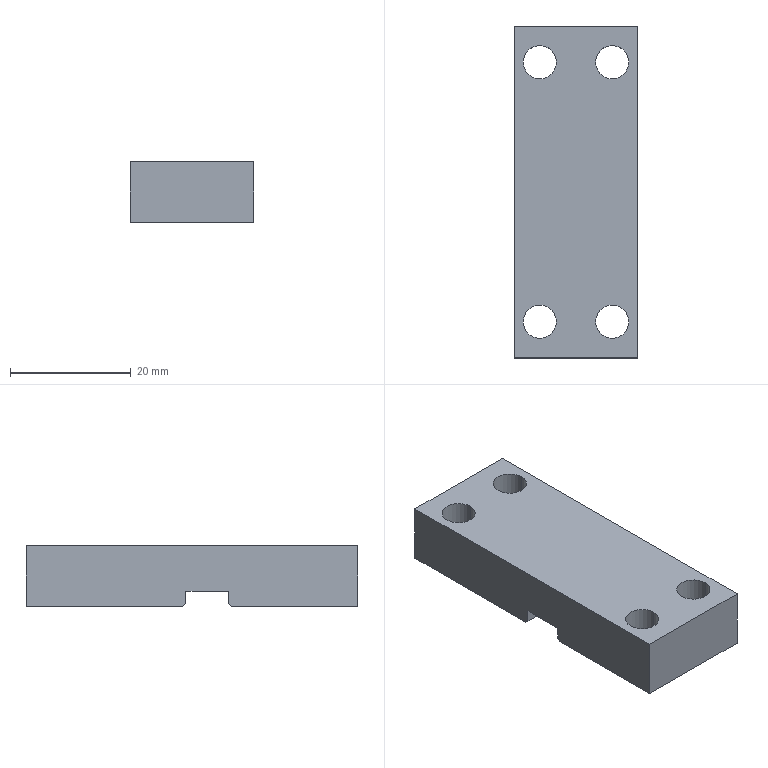Part | STEP file | cover plate 3 | 1 solid | 20 faces | box 20.5 x 55 x 10 mm | volume 9961 mm3 | plane 12 | cylinder 8 | commonest cylinder face diameters 5.5 x8
STEP:
#1=CARTESIAN_POINT('',(0.,0.,0.));
#2=DIRECTION('',(0.,0.,1.));
#3=DIRECTION('',(1.,0.,0.));
#4=AXIS2_PLACEMENT_3D('',#1,#2,#3);
#5=CARTESIAN_POINT('',(3.25,6.,10.));
#6=VERTEX_POINT('',#5);
#7=CARTESIAN_POINT('',(3.25,6.,0.));
#8=VERTEX_POINT('',#7);
#9=CARTESIAN_POINT('',(3.25,6.,10.));
#10=DIRECTION('',(0.,0.,-1.));
#11=VECTOR('',#10,1.);
#12=LINE('',#9,#11);
#13=CARTESIAN_POINT('',(6.,6.,10.));
#14=DIRECTION('',(0.,0.,-1.));
#15=DIRECTION('',(-1.,0.,0.));
#16=AXIS2_PLACEMENT_3D('',#13,#14,#15);
#17=CYLINDRICAL_SURFACE('',#16,2.75);
#18=CARTESIAN_POINT('',(6.283,0.));
#19=DIRECTION('',(0.,1.));
#20=VECTOR('',#19,1.);
#21=LINE('',#18,#20);
#22=(GEOMETRIC_REPRESENTATION_CONTEXT(2)PARAMETRIC_REPRESENTATION_CONTEXT()REPRESENTATION_CONTEXT('',''));
#23=DEFINITIONAL_REPRESENTATION('',(#21),#22);
#24=PCURVE('',#17,#23);
#25=CARTESIAN_POINT('',(6.,6.,10.));
#26=DIRECTION('',(0.,0.,-1.));
#27=DIRECTION('',(-1.,0.,0.));
#28=AXIS2_PLACEMENT_3D('',#25,#26,#27);
#29=CYLINDRICAL_SURFACE('',#28,2.75);
#30=CARTESIAN_POINT('',(0.,0.));
#31=DIRECTION('',(0.,1.));
#32=VECTOR('',#31,1.);
#33=LINE('',#30,#32);
#34=(GEOMETRIC_REPRESENTATION_CONTEXT(2)PARAMETRIC_REPRESENTATION_CONTEXT()REPRESENTATION_CONTEXT('',''));
#35=DEFINITIONAL_REPRESENTATION('',(#33),#34);
#36=PCURVE('',#29,#35);
#37=SURFACE_CURVE('',#12,(#24,#36),.PCURVE_S1.);
#38=EDGE_CURVE('',#6,#8,#37,.T.);
#39=ORIENTED_EDGE('',*,*,#38,.T.);
#40=CARTESIAN_POINT('',(8.75,6.,0.));
#41=VERTEX_POINT('',#40);
#42=CARTESIAN_POINT('',(6.,6.,0.));
#43=DIRECTION('',(0.,0.,1.));
#44=DIRECTION('',(1.,0.,0.));
#45=AXIS2_PLACEMENT_3D('',#42,#43,#44);
#46=CIRCLE('',#45,2.75);
#47=CARTESIAN_POINT('',(9.425,10.));
#48=DIRECTION('',(-1.,0.));
#49=VECTOR('',#48,1.);
#50=LINE('',#47,#49);
#51=(GEOMETRIC_REPRESENTATION_CONTEXT(2)PARAMETRIC_REPRESENTATION_CONTEXT()REPRESENTATION_CONTEXT('',''));
#52=DEFINITIONAL_REPRESENTATION('',(#50),#51);
#53=PCURVE('',#17,#52);
#54=CARTESIAN_POINT('',(-10.25,55.,0.));
#55=DIRECTION('',(0.,0.,1.));
#56=DIRECTION('',(1.,0.,0.));
#57=AXIS2_PLACEMENT_3D('',#54,#55,#56);
#58=PLANE('',#57);
#59=CARTESIAN_POINT('',(16.25,-49.));
#60=DIRECTION('',(1.,0.));
#61=AXIS2_PLACEMENT_2D('',#59,#60);
#62=CIRCLE('',#61,2.75);
#63=(GEOMETRIC_REPRESENTATION_CONTEXT(2)PARAMETRIC_REPRESENTATION_CONTEXT()REPRESENTATION_CONTEXT('',''));
#64=DEFINITIONAL_REPRESENTATION('',(#62),#63);
#65=PCURVE('',#58,#64);
#66=SURFACE_CURVE('',#46,(#53,#65),.PCURVE_S1.);
#67=EDGE_CURVE('',#8,#41,#66,.T.);
#68=ORIENTED_EDGE('',*,*,#67,.T.);
#69=CARTESIAN_POINT('',(8.75,6.,10.));
#70=VERTEX_POINT('',#69);
#71=CARTESIAN_POINT('',(8.75,6.,10.));
#72=DIRECTION('',(0.,0.,-1.));
#73=VECTOR('',#72,1.);
#74=LINE('',#71,#73);
#75=CARTESIAN_POINT('',(3.142,0.));
#76=DIRECTION('',(0.,1.));
#77=VECTOR('',#76,1.);
#78=LINE('',#75,#77);
#79=(GEOMETRIC_REPRESENTATION_CONTEXT(2)PARAMETRIC_REPRESENTATION_CONTEXT()REPRESENTATION_CONTEXT('',''));
#80=DEFINITIONAL_REPRESENTATION('',(#78),#79);
#81=PCURVE('',#17,#80);
#82=CARTESIAN_POINT('',(3.142,0.));
#83=DIRECTION('',(0.,1.));
#84=VECTOR('',#83,1.);
#85=LINE('',#82,#84);
#86=(GEOMETRIC_REPRESENTATION_CONTEXT(2)PARAMETRIC_REPRESENTATION_CONTEXT()REPRESENTATION_CONTEXT('',''));
#87=DEFINITIONAL_REPRESENTATION('',(#85),#86);
#88=PCURVE('',#29,#87);
#89=SURFACE_CURVE('',#74,(#81,#88),.PCURVE_S1.);
#90=EDGE_CURVE('',#70,#41,#89,.T.);
#91=ORIENTED_EDGE('',*,*,#90,.F.);
#92=CARTESIAN_POINT('',(6.,6.,10.));
#93=DIRECTION('',(0.,0.,1.));
#94=DIRECTION('',(1.,0.,0.));
#95=AXIS2_PLACEMENT_3D('',#92,#93,#94);
#96=CIRCLE('',#95,2.75);
#97=CARTESIAN_POINT('',(9.425,0.));
#98=DIRECTION('',(-1.,0.));
#99=VECTOR('',#98,1.);
#100=LINE('',#97,#99);
#101=(GEOMETRIC_REPRESENTATION_CONTEXT(2)PARAMETRIC_REPRESENTATION_CONTEXT()REPRESENTATION_CONTEXT('',''));
#102=DEFINITIONAL_REPRESENTATION('',(#100),#101);
#103=PCURVE('',#17,#102);
#104=CARTESIAN_POINT('',(-10.25,55.,10.));
#105=DIRECTION('',(0.,0.,1.));
#106=DIRECTION('',(1.,0.,0.));
#107=AXIS2_PLACEMENT_3D('',#104,#105,#106);
#108=PLANE('',#107);
#109=CARTESIAN_POINT('',(16.25,-49.));
#110=DIRECTION('',(1.,0.));
#111=AXIS2_PLACEMENT_2D('',#109,#110);
#112=CIRCLE('',#111,2.75);
#113=(GEOMETRIC_REPRESENTATION_CONTEXT(2)PARAMETRIC_REPRESENTATION_CONTEXT()REPRESENTATION_CONTEXT('',''));
#114=DEFINITIONAL_REPRESENTATION('',(#112),#113);
#115=PCURVE('',#108,#114);
#116=SURFACE_CURVE('',#96,(#103,#115),.PCURVE_S1.);
#117=EDGE_CURVE('',#6,#70,#116,.T.);
#118=ORIENTED_EDGE('',*,*,#117,.F.);
#119=EDGE_LOOP('',(#39,#68,#91,#118));
#120=FACE_BOUND('',#119,.F.);
#121=ADVANCED_FACE('',(#120),#17,.F.);
#122=CARTESIAN_POINT('',(-8.75,6.,10.));
#123=VERTEX_POINT('',#122);
#124=CARTESIAN_POINT('',(-8.75,6.,0.));
#125=VERTEX_POINT('',#124);
#126=CARTESIAN_POINT('',(-8.75,6.,10.));
#127=DIRECTION('',(0.,0.,-1.));
#128=VECTOR('',#127,1.);
#129=LINE('',#126,#128);
#130=CARTESIAN_POINT('',(-6.,6.,10.));
#131=DIRECTION('',(0.,0.,-1.));
#132=DIRECTION('',(-1.,0.,0.));
#133=AXIS2_PLACEMENT_3D('',#130,#131,#132);
#134=CYLINDRICAL_SURFACE('',#133,2.75);
#135=CARTESIAN_POINT('',(6.283,0.));
#136=DIRECTION('',(0.,1.));
#137=VECTOR('',#136,1.);
#138=LINE('',#135,#137);
#139=(GEOMETRIC_REPRESENTATION_CONTEXT(2)PARAMETRIC_REPRESENTATION_CONTEXT()REPRESENTATION_CONTEXT('',''));
#140=DEFINITIONAL_REPRESENTATION('',(#138),#139);
#141=PCURVE('',#134,#140);
#142=CARTESIAN_POINT('',(-6.,6.,10.));
#143=DIRECTION('',(0.,0.,-1.));
#144=DIRECTION('',(-1.,0.,0.));
#145=AXIS2_PLACEMENT_3D('',#142,#143,#144);
#146=CYLINDRICAL_SURFACE('',#145,2.75);
#147=CARTESIAN_POINT('',(0.,0.));
#148=DIRECTION('',(0.,1.));
#149=VECTOR('',#148,1.);
#150=LINE('',#147,#149);
#151=(GEOMETRIC_REPRESENTATION_CONTEXT(2)PARAMETRIC_REPRESENTATION_CONTEXT()REPRESENTATION_CONTEXT('',''));
#152=DEFINITIONAL_REPRESENTATION('',(#150),#151);
#153=PCURVE('',#146,#152);
#154=SURFACE_CURVE('',#129,(#141,#153),.PCURVE_S1.);
#155=EDGE_CURVE('',#123,#125,#154,.T.);
#156=ORIENTED_EDGE('',*,*,#155,.T.);
#157=CARTESIAN_POINT('',(-3.25,6.,0.));
#158=VERTEX_POINT('',#157);
#159=CARTESIAN_POINT('',(-6.,6.,0.));
#160=DIRECTION('',(0.,0.,1.));
#161=DIRECTION('',(1.,0.,0.));
#162=AXIS2_PLACEMENT_3D('',#159,#160,#161);
#163=CIRCLE('',#162,2.75);
#164=CARTESIAN_POINT('',(9.425,10.));
#165=DIRECTION('',(-1.,0.));
#166=VECTOR('',#165,1.);
#167=LINE('',#164,#166);
#168=(GEOMETRIC_REPRESENTATION_CONTEXT(2)PARAMETRIC_REPRESENTATION_CONTEXT()REPRESENTATION_CONTEXT('',''));
#169=DEFINITIONAL_REPRESENTATION('',(#167),#168);
#170=PCURVE('',#134,#169);
#171=CARTESIAN_POINT('',(4.25,-49.));
#172=DIRECTION('',(1.,0.));
#173=AXIS2_PLACEMENT_2D('',#171,#172);
#174=CIRCLE('',#173,2.75);
#175=(GEOMETRIC_REPRESENTATION_CONTEXT(2)PARAMETRIC_REPRESENTATION_CONTEXT()REPRESENTATION_CONTEXT('',''));
#176=DEFINITIONAL_REPRESENTATION('',(#174),#175);
#177=PCURVE('',#58,#176);
#178=SURFACE_CURVE('',#163,(#170,#177),.PCURVE_S1.);
#179=EDGE_CURVE('',#125,#158,#178,.T.);
#180=ORIENTED_EDGE('',*,*,#179,.T.);
#181=CARTESIAN_POINT('',(-3.25,6.,10.));
#182=VERTEX_POINT('',#181);
#183=CARTESIAN_POINT('',(-3.25,6.,10.));
#184=DIRECTION('',(0.,0.,-1.));
#185=VECTOR('',#184,1.);
#186=LINE('',#183,#185);
#187=CARTESIAN_POINT('',(3.142,0.));
#188=DIRECTION('',(0.,1.));
#189=VECTOR('',#188,1.);
#190=LINE('',#187,#189);
#191=(GEOMETRIC_REPRESENTATION_CONTEXT(2)PARAMETRIC_REPRESENTATION_CONTEXT()REPRESENTATION_CONTEXT('',''));
#192=DEFINITIONAL_REPRESENTATION('',(#190),#191);
#193=PCURVE('',#134,#192);
#194=CARTESIAN_POINT('',(3.142,0.));
#195=DIRECTION('',(0.,1.));
#196=VECTOR('',#195,1.);
#197=LINE('',#194,#196);
#198=(GEOMETRIC_REPRESENTATION_CONTEXT(2)PARAMETRIC_REPRESENTATION_CONTEXT()REPRESENTATION_CONTEXT('',''));
#199=DEFINITIONAL_REPRESENTATION('',(#197),#198);
#200=PCURVE('',#146,#199);
#201=SURFACE_CURVE('',#186,(#193,#200),.PCURVE_S1.);
#202=EDGE_CURVE('',#182,#158,#201,.T.);
#203=ORIENTED_EDGE('',*,*,#202,.F.);
#204=CARTESIAN_POINT('',(-6.,6.,10.));
#205=DIRECTION('',(0.,0.,1.));
#206=DIRECTION('',(1.,0.,0.));
#207=AXIS2_PLACEMENT_3D('',#204,#205,#206);
#208=CIRCLE('',#207,2.75);
#209=CARTESIAN_POINT('',(9.425,0.));
#210=DIRECTION('',(-1.,0.));
#211=VECTOR('',#210,1.);
#212=LINE('',#209,#211);
#213=(GEOMETRIC_REPRESENTATION_CONTEXT(2)PARAMETRIC_REPRESENTATION_CONTEXT()REPRESENTATION_CONTEXT('',''));
#214=DEFINITIONAL_REPRESENTATION('',(#212),#213);
#215=PCURVE('',#134,#214);
#216=CARTESIAN_POINT('',(4.25,-49.));
#217=DIRECTION('',(1.,0.));
#218=AXIS2_PLACEMENT_2D('',#216,#217);
#219=CIRCLE('',#218,2.75);
#220=(GEOMETRIC_REPRESENTATION_CONTEXT(2)PARAMETRIC_REPRESENTATION_CONTEXT()REPRESENTATION_CONTEXT('',''));
#221=DEFINITIONAL_REPRESENTATION('',(#219),#220);
#222=PCURVE('',#108,#221);
#223=SURFACE_CURVE('',#208,(#215,#222),.PCURVE_S1.);
#224=EDGE_CURVE('',#123,#182,#223,.T.);
#225=ORIENTED_EDGE('',*,*,#224,.F.);
#226=EDGE_LOOP('',(#156,#180,#203,#225));
#227=FACE_BOUND('',#226,.F.);
#228=ADVANCED_FACE('',(#227),#134,.F.);
#229=CARTESIAN_POINT('',(3.25,49.,10.));
#230=VERTEX_POINT('',#229);
#231=CARTESIAN_POINT('',(3.25,49.,0.));
#232=VERTEX_POINT('',#231);
#233=CARTESIAN_POINT('',(3.25,49.,10.));
#234=DIRECTION('',(0.,0.,-1.));
#235=VECTOR('',#234,1.);
#236=LINE('',#233,#235);
#237=CARTESIAN_POINT('',(6.,49.,10.));
#238=DIRECTION('',(0.,0.,-1.));
#239=DIRECTION('',(-1.,0.,0.));
#240=AXIS2_PLACEMENT_3D('',#237,#238,#239);
#241=CYLINDRICAL_SURFACE('',#240,2.75);
#242=CARTESIAN_POINT('',(6.283,0.));
#243=DIRECTION('',(0.,1.));
#244=VECTOR('',#243,1.);
#245=LINE('',#242,#244);
#246=(GEOMETRIC_REPRESENTATION_CONTEXT(2)PARAMETRIC_REPRESENTATION_CONTEXT()REPRESENTATION_CONTEXT('',''));
#247=DEFINITIONAL_REPRESENTATION('',(#245),#246);
#248=PCURVE('',#241,#247);
#249=CARTESIAN_POINT('',(6.,49.,10.));
#250=DIRECTION('',(0.,0.,-1.));
#251=DIRECTION('',(-1.,0.,0.));
#252=AXIS2_PLACEMENT_3D('',#249,#250,#251);
#253=CYLINDRICAL_SURFACE('',#252,2.75);
#254=CARTESIAN_POINT('',(0.,0.));
#255=DIRECTION('',(0.,1.));
#256=VECTOR('',#255,1.);
#257=LINE('',#254,#256);
#258=(GEOMETRIC_REPRESENTATION_CONTEXT(2)PARAMETRIC_REPRESENTATION_CONTEXT()REPRESENTATION_CONTEXT('',''));
#259=DEFINITIONAL_REPRESENTATION('',(#257),#258);
#260=PCURVE('',#253,#259);
#261=SURFACE_CURVE('',#236,(#248,#260),.PCURVE_S1.);
#262=EDGE_CURVE('',#230,#232,#261,.T.);
#263=ORIENTED_EDGE('',*,*,#262,.T.);
#264=CARTESIAN_POINT('',(8.75,49.,0.));
#265=VERTEX_POINT('',#264);
#266=CARTESIAN_POINT('',(6.,49.,0.));
#267=DIRECTION('',(0.,0.,1.));
#268=DIRECTION('',(1.,0.,0.));
#269=AXIS2_PLACEMENT_3D('',#266,#267,#268);
#270=CIRCLE('',#269,2.75);
#271=CARTESIAN_POINT('',(9.425,10.));
#272=DIRECTION('',(-1.,0.));
#273=VECTOR('',#272,1.);
#274=LINE('',#271,#273);
#275=(GEOMETRIC_REPRESENTATION_CONTEXT(2)PARAMETRIC_REPRESENTATION_CONTEXT()REPRESENTATION_CONTEXT('',''));
#276=DEFINITIONAL_REPRESENTATION('',(#274),#275);
#277=PCURVE('',#241,#276);
#278=CARTESIAN_POINT('',(-10.25,55.,0.));
#279=DIRECTION('',(0.,0.,1.));
#280=DIRECTION('',(1.,0.,0.));
#281=AXIS2_PLACEMENT_3D('',#278,#279,#280);
#282=PLANE('',#281);
#283=CARTESIAN_POINT('',(16.25,-6.));
#284=DIRECTION('',(1.,0.));
#285=AXIS2_PLACEMENT_2D('',#283,#284);
#286=CIRCLE('',#285,2.75);
#287=(GEOMETRIC_REPRESENTATION_CONTEXT(2)PARAMETRIC_REPRESENTATION_CONTEXT()REPRESENTATION_CONTEXT('',''));
#288=DEFINITIONAL_REPRESENTATION('',(#286),#287);
#289=PCURVE('',#282,#288);
#290=SURFACE_CURVE('',#270,(#277,#289),.PCURVE_S1.);
#291=EDGE_CURVE('',#232,#265,#290,.T.);
#292=ORIENTED_EDGE('',*,*,#291,.T.);
#293=CARTESIAN_POINT('',(8.75,49.,10.));
#294=VERTEX_POINT('',#293);
#295=CARTESIAN_POINT('',(8.75,49.,10.));
#296=DIRECTION('',(0.,0.,-1.));
#297=VECTOR('',#296,1.);
#298=LINE('',#295,#297);
#299=CARTESIAN_POINT('',(3.142,0.));
#300=DIRECTION('',(0.,1.));
#301=VECTOR('',#300,1.);
#302=LINE('',#299,#301);
#303=(GEOMETRIC_REPRESENTATION_CONTEXT(2)PARAMETRIC_REPRESENTATION_CONTEXT()REPRESENTATION_CONTEXT('',''));
#304=DEFINITIONAL_REPRESENTATION('',(#302),#303);
#305=PCURVE('',#241,#304);
#306=CARTESIAN_POINT('',(3.142,0.));
#307=DIRECTION('',(0.,1.));
#308=VECTOR('',#307,1.);
#309=LINE('',#306,#308);
#310=(GEOMETRIC_REPRESENTATION_CONTEXT(2)PARAMETRIC_REPRESENTATION_CONTEXT()REPRESENTATION_CONTEXT('',''));
#311=DEFINITIONAL_REPRESENTATION('',(#309),#310);
#312=PCURVE('',#253,#311);
#313=SURFACE_CURVE('',#298,(#305,#312),.PCURVE_S1.);
#314=EDGE_CURVE('',#294,#265,#313,.T.);
#315=ORIENTED_EDGE('',*,*,#314,.F.);
#316=CARTESIAN_POINT('',(6.,49.,10.));
#317=DIRECTION('',(0.,0.,1.));
#318=DIRECTION('',(1.,0.,0.));
#319=AXIS2_PLACEMENT_3D('',#316,#317,#318);
#320=CIRCLE('',#319,2.75);
#321=CARTESIAN_POINT('',(9.425,0.));
#322=DIRECTION('',(-1.,0.));
#323=VECTOR('',#322,1.);
#324=LINE('',#321,#323);
#325=(GEOMETRIC_REPRESENTATION_CONTEXT(2)PARAMETRIC_REPRESENTATION_CONTEXT()REPRESENTATION_CONTEXT('',''));
#326=DEFINITIONAL_REPRESENTATION('',(#324),#325);
#327=PCURVE('',#241,#326);
#328=CARTESIAN_POINT('',(16.25,-6.));
#329=DIRECTION('',(1.,0.));
#330=AXIS2_PLACEMENT_2D('',#328,#329);
#331=CIRCLE('',#330,2.75);
#332=(GEOMETRIC_REPRESENTATION_CONTEXT(2)PARAMETRIC_REPRESENTATION_CONTEXT()REPRESENTATION_CONTEXT('',''));
#333=DEFINITIONAL_REPRESENTATION('',(#331),#332);
#334=PCURVE('',#108,#333);
#335=SURFACE_CURVE('',#320,(#327,#334),.PCURVE_S1.);
#336=EDGE_CURVE('',#230,#294,#335,.T.);
#337=ORIENTED_EDGE('',*,*,#336,.F.);
#338=EDGE_LOOP('',(#263,#292,#315,#337));
#339=FACE_BOUND('',#338,.F.);
#340=ADVANCED_FACE('',(#339),#241,.F.);
#341=CARTESIAN_POINT('',(-8.75,49.,10.));
#342=VERTEX_POINT('',#341);
#343=CARTESIAN_POINT('',(-8.75,49.,0.));
#344=VERTEX_POINT('',#343);
#345=CARTESIAN_POINT('',(-8.75,49.,10.));
#346=DIRECTION('',(0.,0.,-1.));
#347=VECTOR('',#346,1.);
#348=LINE('',#345,#347);
#349=CARTESIAN_POINT('',(-6.,49.,10.));
#350=DIRECTION('',(0.,0.,-1.));
#351=DIRECTION('',(-1.,0.,0.));
#352=AXIS2_PLACEMENT_3D('',#349,#350,#351);
#353=CYLINDRICAL_SURFACE('',#352,2.75);
#354=CARTESIAN_POINT('',(6.283,0.));
#355=DIRECTION('',(0.,1.));
#356=VECTOR('',#355,1.);
#357=LINE('',#354,#356);
#358=(GEOMETRIC_REPRESENTATION_CONTEXT(2)PARAMETRIC_REPRESENTATION_CONTEXT()REPRESENTATION_CONTEXT('',''));
#359=DEFINITIONAL_REPRESENTATION('',(#357),#358);
#360=PCURVE('',#353,#359);
#361=CARTESIAN_POINT('',(-6.,49.,10.));
#362=DIRECTION('',(0.,0.,-1.));
#363=DIRECTION('',(-1.,0.,0.));
#364=AXIS2_PLACEMENT_3D('',#361,#362,#363);
#365=CYLINDRICAL_SURFACE('',#364,2.75);
#366=CARTESIAN_POINT('',(0.,0.));
#367=DIRECTION('',(0.,1.));
#368=VECTOR('',#367,1.);
#369=LINE('',#366,#368);
#370=(GEOMETRIC_REPRESENTATION_CONTEXT(2)PARAMETRIC_REPRESENTATION_CONTEXT()REPRESENTATION_CONTEXT('',''));
#371=DEFINITIONAL_REPRESENTATION('',(#369),#370);
#372=PCURVE('',#365,#371);
#373=SURFACE_CURVE('',#348,(#360,#372),.PCURVE_S1.);
#374=EDGE_CURVE('',#342,#344,#373,.T.);
#375=ORIENTED_EDGE('',*,*,#374,.T.);
#376=CARTESIAN_POINT('',(-3.25,49.,0.));
#377=VERTEX_POINT('',#376);
#378=CARTESIAN_POINT('',(-6.,49.,0.));
#379=DIRECTION('',(0.,0.,1.));
#380=DIRECTION('',(1.,0.,0.));
#381=AXIS2_PLACEMENT_3D('',#378,#379,#380);
#382=CIRCLE('',#381,2.75);
#383=CARTESIAN_POINT('',(9.425,10.));
#384=DIRECTION('',(-1.,0.));
#385=VECTOR('',#384,1.);
#386=LINE('',#383,#385);
#387=(GEOMETRIC_REPRESENTATION_CONTEXT(2)PARAMETRIC_REPRESENTATION_CONTEXT()REPRESENTATION_CONTEXT('',''));
#388=DEFINITIONAL_REPRESENTATION('',(#386),#387);
#389=PCURVE('',#353,#388);
#390=CARTESIAN_POINT('',(4.25,-6.));
#391=DIRECTION('',(1.,0.));
#392=AXIS2_PLACEMENT_2D('',#390,#391);
#393=CIRCLE('',#392,2.75);
#394=(GEOMETRIC_REPRESENTATION_CONTEXT(2)PARAMETRIC_REPRESENTATION_CONTEXT()REPRESENTATION_CONTEXT('',''));
#395=DEFINITIONAL_REPRESENTATION('',(#393),#394);
#396=PCURVE('',#282,#395);
#397=SURFACE_CURVE('',#382,(#389,#396),.PCURVE_S1.);
#398=EDGE_CURVE('',#344,#377,#397,.T.);
#399=ORIENTED_EDGE('',*,*,#398,.T.);
#400=CARTESIAN_POINT('',(-3.25,49.,10.));
#401=VERTEX_POINT('',#400);
#402=CARTESIAN_POINT('',(-3.25,49.,10.));
#403=DIRECTION('',(0.,0.,-1.));
#404=VECTOR('',#403,1.);
#405=LINE('',#402,#404);
#406=CARTESIAN_POINT('',(3.142,0.));
#407=DIRECTION('',(0.,1.));
#408=VECTOR('',#407,1.);
#409=LINE('',#406,#408);
#410=(GEOMETRIC_REPRESENTATION_CONTEXT(2)PARAMETRIC_REPRESENTATION_CONTEXT()REPRESENTATION_CONTEXT('',''));
#411=DEFINITIONAL_REPRESENTATION('',(#409),#410);
#412=PCURVE('',#353,#411);
#413=CARTESIAN_POINT('',(3.142,0.));
#414=DIRECTION('',(0.,1.));
#415=VECTOR('',#414,1.);
#416=LINE('',#413,#415);
#417=(GEOMETRIC_REPRESENTATION_CONTEXT(2)PARAMETRIC_REPRESENTATION_CONTEXT()REPRESENTATION_CONTEXT('',''));
#418=DEFINITIONAL_REPRESENTATION('',(#416),#417);
#419=PCURVE('',#365,#418);
#420=SURFACE_CURVE('',#405,(#412,#419),.PCURVE_S1.);
#421=EDGE_CURVE('',#401,#377,#420,.T.);
#422=ORIENTED_EDGE('',*,*,#421,.F.);
#423=CARTESIAN_POINT('',(-6.,49.,10.));
#424=DIRECTION('',(0.,0.,1.));
#425=DIRECTION('',(1.,0.,0.));
#426=AXIS2_PLACEMENT_3D('',#423,#424,#425);
#427=CIRCLE('',#426,2.75);
#428=CARTESIAN_POINT('',(9.425,0.));
#429=DIRECTION('',(-1.,0.));
#430=VECTOR('',#429,1.);
#431=LINE('',#428,#430);
#432=(GEOMETRIC_REPRESENTATION_CONTEXT(2)PARAMETRIC_REPRESENTATION_CONTEXT()REPRESENTATION_CONTEXT('',''));
#433=DEFINITIONAL_REPRESENTATION('',(#431),#432);
#434=PCURVE('',#353,#433);
#435=CARTESIAN_POINT('',(4.25,-6.));
#436=DIRECTION('',(1.,0.));
#437=AXIS2_PLACEMENT_2D('',#435,#436);
#438=CIRCLE('',#437,2.75);
#439=(GEOMETRIC_REPRESENTATION_CONTEXT(2)PARAMETRIC_REPRESENTATION_CONTEXT()REPRESENTATION_CONTEXT('',''));
#440=DEFINITIONAL_REPRESENTATION('',(#438),#439);
#441=PCURVE('',#108,#440);
#442=SURFACE_CURVE('',#427,(#434,#441),.PCURVE_S1.);
#443=EDGE_CURVE('',#342,#401,#442,.T.);
#444=ORIENTED_EDGE('',*,*,#443,.F.);
#445=EDGE_LOOP('',(#375,#399,#422,#444));
#446=FACE_BOUND('',#445,.F.);
#447=ADVANCED_FACE('',(#446),#353,.F.);
#448=ORIENTED_EDGE('',*,*,#291,.T.);
#449=CARTESIAN_POINT('',(6.,49.,0.));
#450=DIRECTION('',(0.,0.,1.));
#451=DIRECTION('',(1.,0.,0.));
#452=AXIS2_PLACEMENT_3D('',#449,#450,#451);
#453=CIRCLE('',#452,2.75);
#454=CARTESIAN_POINT('',(16.25,-6.));
#455=DIRECTION('',(1.,0.));
#456=AXIS2_PLACEMENT_2D('',#454,#455);
#457=CIRCLE('',#456,2.75);
#458=(GEOMETRIC_REPRESENTATION_CONTEXT(2)PARAMETRIC_REPRESENTATION_CONTEXT()REPRESENTATION_CONTEXT('',''));
#459=DEFINITIONAL_REPRESENTATION('',(#457),#458);
#460=PCURVE('',#282,#459);
#461=CARTESIAN_POINT('',(3.142,10.));
#462=DIRECTION('',(-1.,0.));
#463=VECTOR('',#462,1.);
#464=LINE('',#461,#463);
#465=(GEOMETRIC_REPRESENTATION_CONTEXT(2)PARAMETRIC_REPRESENTATION_CONTEXT()REPRESENTATION_CONTEXT('',''));
#466=DEFINITIONAL_REPRESENTATION('',(#464),#465);
#467=PCURVE('',#253,#466);
#468=SURFACE_CURVE('',#453,(#460,#467),.PCURVE_S1.);
#469=EDGE_CURVE('',#265,#232,#468,.T.);
#470=ORIENTED_EDGE('',*,*,#469,.T.);
#471=EDGE_LOOP('',(#448,#470));
#472=FACE_BOUND('',#471,.T.);
#473=ORIENTED_EDGE('',*,*,#398,.T.);
#474=CARTESIAN_POINT('',(-6.,49.,0.));
#475=DIRECTION('',(0.,0.,1.));
#476=DIRECTION('',(1.,0.,0.));
#477=AXIS2_PLACEMENT_3D('',#474,#475,#476);
#478=CIRCLE('',#477,2.75);
#479=CARTESIAN_POINT('',(4.25,-6.));
#480=DIRECTION('',(1.,0.));
#481=AXIS2_PLACEMENT_2D('',#479,#480);
#482=CIRCLE('',#481,2.75);
#483=(GEOMETRIC_REPRESENTATION_CONTEXT(2)PARAMETRIC_REPRESENTATION_CONTEXT()REPRESENTATION_CONTEXT('',''));
#484=DEFINITIONAL_REPRESENTATION('',(#482),#483);
#485=PCURVE('',#282,#484);
#486=CARTESIAN_POINT('',(3.142,10.));
#487=DIRECTION('',(-1.,0.));
#488=VECTOR('',#487,1.);
#489=LINE('',#486,#488);
#490=(GEOMETRIC_REPRESENTATION_CONTEXT(2)PARAMETRIC_REPRESENTATION_CONTEXT()REPRESENTATION_CONTEXT('',''));
#491=DEFINITIONAL_REPRESENTATION('',(#489),#490);
#492=PCURVE('',#365,#491);
#493=SURFACE_CURVE('',#478,(#485,#492),.PCURVE_S1.);
#494=EDGE_CURVE('',#377,#344,#493,.T.);
#495=ORIENTED_EDGE('',*,*,#494,.T.);
#496=EDGE_LOOP('',(#473,#495));
#497=FACE_BOUND('',#496,.T.);
#498=CARTESIAN_POINT('',(10.25,29.,0.));
#499=VERTEX_POINT('',#498);
#500=CARTESIAN_POINT('',(10.25,55.,0.));
#501=VERTEX_POINT('',#500);
#502=CARTESIAN_POINT('',(10.25,55.,0.));
#503=DIRECTION('',(0.,1.,0.));
#504=VECTOR('',#503,1.);
#505=LINE('',#502,#504);
#506=CARTESIAN_POINT('',(20.5,0.));
#507=DIRECTION('',(0.,1.));
#508=VECTOR('',#507,1.);
#509=LINE('',#506,#508);
#510=(GEOMETRIC_REPRESENTATION_CONTEXT(2)PARAMETRIC_REPRESENTATION_CONTEXT()REPRESENTATION_CONTEXT('',''));
#511=DEFINITIONAL_REPRESENTATION('',(#509),#510);
#512=PCURVE('',#282,#511);
#513=CARTESIAN_POINT('',(10.25,55.,10.));
#514=DIRECTION('',(-1.,0.,0.));
#515=DIRECTION('',(0.,-1.,0.));
#516=AXIS2_PLACEMENT_3D('',#513,#514,#515);
#517=PLANE('',#516);
#518=CARTESIAN_POINT('',(0.,-10.));
#519=DIRECTION('',(-1.,0.));
#520=VECTOR('',#519,1.);
#521=LINE('',#518,#520);
#522=(GEOMETRIC_REPRESENTATION_CONTEXT(2)PARAMETRIC_REPRESENTATION_CONTEXT()REPRESENTATION_CONTEXT('',''));
#523=DEFINITIONAL_REPRESENTATION('',(#521),#522);
#524=PCURVE('',#517,#523);
#525=SURFACE_CURVE('',#505,(#512,#524),.PCURVE_S1.);
#526=EDGE_CURVE('',#499,#501,#525,.T.);
#527=ORIENTED_EDGE('',*,*,#526,.F.);
#528=CARTESIAN_POINT('',(-10.25,29.,0.));
#529=VERTEX_POINT('',#528);
#530=CARTESIAN_POINT('',(-10.25,29.,0.));
#531=DIRECTION('',(-1.,0.,0.));
#532=VECTOR('',#531,1.);
#533=LINE('',#530,#532);
#534=CARTESIAN_POINT('',(0.,-26.));
#535=DIRECTION('',(-1.,0.));
#536=VECTOR('',#535,1.);
#537=LINE('',#534,#536);
#538=(GEOMETRIC_REPRESENTATION_CONTEXT(2)PARAMETRIC_REPRESENTATION_CONTEXT()REPRESENTATION_CONTEXT('',''));
#539=DEFINITIONAL_REPRESENTATION('',(#537),#538);
#540=PCURVE('',#282,#539);
#541=CARTESIAN_POINT('',(-10.25,29.,0.));
#542=DIRECTION('',(0.,0.7071,0.7071));
#543=DIRECTION('',(0.,-0.7071,0.7071));
#544=AXIS2_PLACEMENT_3D('',#541,#542,#543);
#545=PLANE('',#544);
#546=CARTESIAN_POINT('',(0.,0.));
#547=DIRECTION('',(0.,-1.));
#548=VECTOR('',#547,1.);
#549=LINE('',#546,#548);
#550=(GEOMETRIC_REPRESENTATION_CONTEXT(2)PARAMETRIC_REPRESENTATION_CONTEXT()REPRESENTATION_CONTEXT('',''));
#551=DEFINITIONAL_REPRESENTATION('',(#549),#550);
#552=PCURVE('',#545,#551);
#553=SURFACE_CURVE('',#533,(#540,#552),.PCURVE_S1.);
#554=EDGE_CURVE('',#499,#529,#553,.T.);
#555=ORIENTED_EDGE('',*,*,#554,.T.);
#556=CARTESIAN_POINT('',(-10.25,55.,0.));
#557=VERTEX_POINT('',#556);
#558=CARTESIAN_POINT('',(-10.25,0.5,0.));
#559=DIRECTION('',(0.,-1.,0.));
#560=VECTOR('',#559,1.);
#561=LINE('',#558,#560);
#562=CARTESIAN_POINT('',(0.,-54.5));
#563=DIRECTION('',(0.,-1.));
#564=VECTOR('',#563,1.);
#565=LINE('',#562,#564);
#566=(GEOMETRIC_REPRESENTATION_CONTEXT(2)PARAMETRIC_REPRESENTATION_CONTEXT()REPRESENTATION_CONTEXT('',''));
#567=DEFINITIONAL_REPRESENTATION('',(#565),#566);
#568=PCURVE('',#282,#567);
#569=CARTESIAN_POINT('',(-10.25,0.5,10.));
#570=DIRECTION('',(1.,0.,0.));
#571=DIRECTION('',(0.,0.,-1.));
#572=AXIS2_PLACEMENT_3D('',#569,#570,#571);
#573=PLANE('',#572);
#574=CARTESIAN_POINT('',(10.,0.));
#575=DIRECTION('',(0.,-1.));
#576=VECTOR('',#575,1.);
#577=LINE('',#574,#576);
#578=(GEOMETRIC_REPRESENTATION_CONTEXT(2)PARAMETRIC_REPRESENTATION_CONTEXT()REPRESENTATION_CONTEXT('',''));
#579=DEFINITIONAL_REPRESENTATION('',(#577),#578);
#580=PCURVE('',#573,#579);
#581=SURFACE_CURVE('',#561,(#568,#580),.PCURVE_S1.);
#582=EDGE_CURVE('',#557,#529,#581,.T.);
#583=ORIENTED_EDGE('',*,*,#582,.F.);
#584=CARTESIAN_POINT('',(-10.25,55.,0.));
#585=DIRECTION('',(-1.,0.,0.));
#586=VECTOR('',#585,1.);
#587=LINE('',#584,#586);
#588=CARTESIAN_POINT('',(0.,0.));
#589=DIRECTION('',(-1.,0.));
#590=VECTOR('',#589,1.);
#591=LINE('',#588,#590);
#592=(GEOMETRIC_REPRESENTATION_CONTEXT(2)PARAMETRIC_REPRESENTATION_CONTEXT()REPRESENTATION_CONTEXT('',''));
#593=DEFINITIONAL_REPRESENTATION('',(#591),#592);
#594=PCURVE('',#282,#593);
#595=CARTESIAN_POINT('',(-10.25,55.,10.));
#596=DIRECTION('',(0.,-1.,0.));
#597=DIRECTION('',(0.,0.,-1.));
#598=AXIS2_PLACEMENT_3D('',#595,#596,#597);
#599=PLANE('',#598);
#600=CARTESIAN_POINT('',(10.,0.));
#601=DIRECTION('',(0.,-1.));
#602=VECTOR('',#601,1.);
#603=LINE('',#600,#602);
#604=(GEOMETRIC_REPRESENTATION_CONTEXT(2)PARAMETRIC_REPRESENTATION_CONTEXT()REPRESENTATION_CONTEXT('',''));
#605=DEFINITIONAL_REPRESENTATION('',(#603),#604);
#606=PCURVE('',#599,#605);
#607=SURFACE_CURVE('',#587,(#594,#606),.PCURVE_S1.);
#608=EDGE_CURVE('',#501,#557,#607,.T.);
#609=ORIENTED_EDGE('',*,*,#608,.F.);
#610=EDGE_LOOP('',(#527,#555,#583,#609));
#611=FACE_BOUND('',#610,.T.);
#612=ADVANCED_FACE('',(#472,#497,#611),#282,.F.);
#613=ORIENTED_EDGE('',*,*,#224,.F.);
#614=CARTESIAN_POINT('',(-6.,6.,10.));
#615=DIRECTION('',(0.,0.,1.));
#616=DIRECTION('',(1.,0.,0.));
#617=AXIS2_PLACEMENT_3D('',#614,#615,#616);
#618=CIRCLE('',#617,2.75);
#619=CARTESIAN_POINT('',(4.25,-49.));
#620=DIRECTION('',(1.,0.));
#621=AXIS2_PLACEMENT_2D('',#619,#620);
#622=CIRCLE('',#621,2.75);
#623=(GEOMETRIC_REPRESENTATION_CONTEXT(2)PARAMETRIC_REPRESENTATION_CONTEXT()REPRESENTATION_CONTEXT('',''));
#624=DEFINITIONAL_REPRESENTATION('',(#622),#623);
#625=PCURVE('',#108,#624);
#626=CARTESIAN_POINT('',(3.142,0.));
#627=DIRECTION('',(-1.,0.));
#628=VECTOR('',#627,1.);
#629=LINE('',#626,#628);
#630=(GEOMETRIC_REPRESENTATION_CONTEXT(2)PARAMETRIC_REPRESENTATION_CONTEXT()REPRESENTATION_CONTEXT('',''));
#631=DEFINITIONAL_REPRESENTATION('',(#629),#630);
#632=PCURVE('',#146,#631);
#633=SURFACE_CURVE('',#618,(#625,#632),.PCURVE_S1.);
#634=EDGE_CURVE('',#182,#123,#633,.T.);
#635=ORIENTED_EDGE('',*,*,#634,.F.);
#636=EDGE_LOOP('',(#613,#635));
#637=FACE_BOUND('',#636,.T.);
#638=ORIENTED_EDGE('',*,*,#443,.F.);
#639=CARTESIAN_POINT('',(-6.,49.,10.));
#640=DIRECTION('',(0.,0.,1.));
#641=DIRECTION('',(1.,0.,0.));
#642=AXIS2_PLACEMENT_3D('',#639,#640,#641);
#643=CIRCLE('',#642,2.75);
#644=CARTESIAN_POINT('',(4.25,-6.));
#645=DIRECTION('',(1.,0.));
#646=AXIS2_PLACEMENT_2D('',#644,#645);
#647=CIRCLE('',#646,2.75);
#648=(GEOMETRIC_REPRESENTATION_CONTEXT(2)PARAMETRIC_REPRESENTATION_CONTEXT()REPRESENTATION_CONTEXT('',''));
#649=DEFINITIONAL_REPRESENTATION('',(#647),#648);
#650=PCURVE('',#108,#649);
#651=CARTESIAN_POINT('',(3.142,0.));
#652=DIRECTION('',(-1.,0.));
#653=VECTOR('',#652,1.);
#654=LINE('',#651,#653);
#655=(GEOMETRIC_REPRESENTATION_CONTEXT(2)PARAMETRIC_REPRESENTATION_CONTEXT()REPRESENTATION_CONTEXT('',''));
#656=DEFINITIONAL_REPRESENTATION('',(#654),#655);
#657=PCURVE('',#365,#656);
#658=SURFACE_CURVE('',#643,(#650,#657),.PCURVE_S1.);
#659=EDGE_CURVE('',#401,#342,#658,.T.);
#660=ORIENTED_EDGE('',*,*,#659,.F.);
#661=EDGE_LOOP('',(#638,#660));
#662=FACE_BOUND('',#661,.T.);
#663=CARTESIAN_POINT('',(-10.25,55.,10.));
#664=VERTEX_POINT('',#663);
#665=CARTESIAN_POINT('',(-10.25,0.,10.));
#666=VERTEX_POINT('',#665);
#667=CARTESIAN_POINT('',(-10.25,0.5,10.));
#668=DIRECTION('',(0.,-1.,0.));
#669=VECTOR('',#668,1.);
#670=LINE('',#667,#669);
#671=CARTESIAN_POINT('',(0.,-54.5));
#672=DIRECTION('',(0.,-1.));
#673=VECTOR('',#672,1.);
#674=LINE('',#671,#673);
#675=(GEOMETRIC_REPRESENTATION_CONTEXT(2)PARAMETRIC_REPRESENTATION_CONTEXT()REPRESENTATION_CONTEXT('',''));
#676=DEFINITIONAL_REPRESENTATION('',(#674),#675);
#677=PCURVE('',#108,#676);
#678=CARTESIAN_POINT('',(0.,0.));
#679=DIRECTION('',(0.,-1.));
#680=VECTOR('',#679,1.);
#681=LINE('',#678,#680);
#682=(GEOMETRIC_REPRESENTATION_CONTEXT(2)PARAMETRIC_REPRESENTATION_CONTEXT()REPRESENTATION_CONTEXT('',''));
#683=DEFINITIONAL_REPRESENTATION('',(#681),#682);
#684=PCURVE('',#573,#683);
#685=SURFACE_CURVE('',#670,(#677,#684),.PCURVE_S1.);
#686=EDGE_CURVE('',#664,#666,#685,.T.);
#687=ORIENTED_EDGE('',*,*,#686,.T.);
#688=CARTESIAN_POINT('',(10.25,0.,10.));
#689=VERTEX_POINT('',#688);
#690=CARTESIAN_POINT('',(10.25,0.,10.));
#691=DIRECTION('',(1.,0.,0.));
#692=VECTOR('',#691,1.);
#693=LINE('',#690,#692);
#694=CARTESIAN_POINT('',(20.5,-55.));
#695=DIRECTION('',(1.,0.));
#696=VECTOR('',#695,1.);
#697=LINE('',#694,#696);
#698=(GEOMETRIC_REPRESENTATION_CONTEXT(2)PARAMETRIC_REPRESENTATION_CONTEXT()REPRESENTATION_CONTEXT('',''));
#699=DEFINITIONAL_REPRESENTATION('',(#697),#698);
#700=PCURVE('',#108,#699);
#701=CARTESIAN_POINT('',(10.25,0.,10.));
#702=DIRECTION('',(0.,1.,0.));
#703=DIRECTION('',(-1.,0.,0.));
#704=AXIS2_PLACEMENT_3D('',#701,#702,#703);
#705=PLANE('',#704);
#706=CARTESIAN_POINT('',(0.,0.));
#707=DIRECTION('',(-1.,0.));
#708=VECTOR('',#707,1.);
#709=LINE('',#706,#708);
#710=(GEOMETRIC_REPRESENTATION_CONTEXT(2)PARAMETRIC_REPRESENTATION_CONTEXT()REPRESENTATION_CONTEXT('',''));
#711=DEFINITIONAL_REPRESENTATION('',(#709),#710);
#712=PCURVE('',#705,#711);
#713=SURFACE_CURVE('',#693,(#700,#712),.PCURVE_S1.);
#714=EDGE_CURVE('',#666,#689,#713,.T.);
#715=ORIENTED_EDGE('',*,*,#714,.T.);
#716=CARTESIAN_POINT('',(10.25,55.,10.));
#717=VERTEX_POINT('',#716);
#718=CARTESIAN_POINT('',(10.25,0.5,10.));
#719=DIRECTION('',(0.,1.,0.));
#720=VECTOR('',#719,1.);
#721=LINE('',#718,#720);
#722=CARTESIAN_POINT('',(20.5,-54.5));
#723=DIRECTION('',(0.,1.));
#724=VECTOR('',#723,1.);
#725=LINE('',#722,#724);
#726=(GEOMETRIC_REPRESENTATION_CONTEXT(2)PARAMETRIC_REPRESENTATION_CONTEXT()REPRESENTATION_CONTEXT('',''));
#727=DEFINITIONAL_REPRESENTATION('',(#725),#726);
#728=PCURVE('',#108,#727);
#729=CARTESIAN_POINT('',(54.5,0.));
#730=DIRECTION('',(-1.,0.));
#731=VECTOR('',#730,1.);
#732=LINE('',#729,#731);
#733=(GEOMETRIC_REPRESENTATION_CONTEXT(2)PARAMETRIC_REPRESENTATION_CONTEXT()REPRESENTATION_CONTEXT('',''));
#734=DEFINITIONAL_REPRESENTATION('',(#732),#733);
#735=PCURVE('',#517,#734);
#736=SURFACE_CURVE('',#721,(#728,#735),.PCURVE_S1.);
#737=EDGE_CURVE('',#689,#717,#736,.T.);
#738=ORIENTED_EDGE('',*,*,#737,.T.);
#739=CARTESIAN_POINT('',(9.75,55.,10.));
#740=DIRECTION('',(-1.,0.,0.));
#741=VECTOR('',#740,1.);
#742=LINE('',#739,#741);
#743=CARTESIAN_POINT('',(20.,0.));
#744=DIRECTION('',(-1.,0.));
#745=VECTOR('',#744,1.);
#746=LINE('',#743,#745);
#747=(GEOMETRIC_REPRESENTATION_CONTEXT(2)PARAMETRIC_REPRESENTATION_CONTEXT()REPRESENTATION_CONTEXT('',''));
#748=DEFINITIONAL_REPRESENTATION('',(#746),#747);
#749=PCURVE('',#108,#748);
#750=CARTESIAN_POINT('',(0.,20.));
#751=DIRECTION('',(0.,-1.));
#752=VECTOR('',#751,1.);
#753=LINE('',#750,#752);
#754=(GEOMETRIC_REPRESENTATION_CONTEXT(2)PARAMETRIC_REPRESENTATION_CONTEXT()REPRESENTATION_CONTEXT('',''));
#755=DEFINITIONAL_REPRESENTATION('',(#753),#754);
#756=PCURVE('',#599,#755);
#757=SURFACE_CURVE('',#742,(#749,#756),.PCURVE_S1.);
#758=EDGE_CURVE('',#717,#664,#757,.T.);
#759=ORIENTED_EDGE('',*,*,#758,.T.);
#760=EDGE_LOOP('',(#687,#715,#738,#759));
#761=FACE_BOUND('',#760,.T.);
#762=ORIENTED_EDGE('',*,*,#336,.F.);
#763=CARTESIAN_POINT('',(6.,49.,10.));
#764=DIRECTION('',(0.,0.,1.));
#765=DIRECTION('',(1.,0.,0.));
#766=AXIS2_PLACEMENT_3D('',#763,#764,#765);
#767=CIRCLE('',#766,2.75);
#768=CARTESIAN_POINT('',(16.25,-6.));
#769=DIRECTION('',(1.,0.));
#770=AXIS2_PLACEMENT_2D('',#768,#769);
#771=CIRCLE('',#770,2.75);
#772=(GEOMETRIC_REPRESENTATION_CONTEXT(2)PARAMETRIC_REPRESENTATION_CONTEXT()REPRESENTATION_CONTEXT('',''));
#773=DEFINITIONAL_REPRESENTATION('',(#771),#772);
#774=PCURVE('',#108,#773);
#775=CARTESIAN_POINT('',(3.142,0.));
#776=DIRECTION('',(-1.,0.));
#777=VECTOR('',#776,1.);
#778=LINE('',#775,#777);
#779=(GEOMETRIC_REPRESENTATION_CONTEXT(2)PARAMETRIC_REPRESENTATION_CONTEXT()REPRESENTATION_CONTEXT('',''));
#780=DEFINITIONAL_REPRESENTATION('',(#778),#779);
#781=PCURVE('',#253,#780);
#782=SURFACE_CURVE('',#767,(#774,#781),.PCURVE_S1.);
#783=EDGE_CURVE('',#294,#230,#782,.T.);
#784=ORIENTED_EDGE('',*,*,#783,.F.);
#785=EDGE_LOOP('',(#762,#784));
#786=FACE_BOUND('',#785,.T.);
#787=ORIENTED_EDGE('',*,*,#117,.F.);
#788=CARTESIAN_POINT('',(6.,6.,10.));
#789=DIRECTION('',(0.,0.,1.));
#790=DIRECTION('',(1.,0.,0.));
#791=AXIS2_PLACEMENT_3D('',#788,#789,#790);
#792=CIRCLE('',#791,2.75);
#793=CARTESIAN_POINT('',(16.25,-49.));
#794=DIRECTION('',(1.,0.));
#795=AXIS2_PLACEMENT_2D('',#793,#794);
#796=CIRCLE('',#795,2.75);
#797=(GEOMETRIC_REPRESENTATION_CONTEXT(2)PARAMETRIC_REPRESENTATION_CONTEXT()REPRESENTATION_CONTEXT('',''));
#798=DEFINITIONAL_REPRESENTATION('',(#796),#797);
#799=PCURVE('',#108,#798);
#800=CARTESIAN_POINT('',(3.142,0.));
#801=DIRECTION('',(-1.,0.));
#802=VECTOR('',#801,1.);
#803=LINE('',#800,#802);
#804=(GEOMETRIC_REPRESENTATION_CONTEXT(2)PARAMETRIC_REPRESENTATION_CONTEXT()REPRESENTATION_CONTEXT('',''));
#805=DEFINITIONAL_REPRESENTATION('',(#803),#804);
#806=PCURVE('',#29,#805);
#807=SURFACE_CURVE('',#792,(#799,#806),.PCURVE_S1.);
#808=EDGE_CURVE('',#70,#6,#807,.T.);
#809=ORIENTED_EDGE('',*,*,#808,.F.);
#810=EDGE_LOOP('',(#787,#809));
#811=FACE_BOUND('',#810,.T.);
#812=ADVANCED_FACE('',(#637,#662,#761,#786,#811),#108,.T.);
#813=ORIENTED_EDGE('',*,*,#179,.T.);
#814=CARTESIAN_POINT('',(-6.,6.,0.));
#815=DIRECTION('',(0.,0.,1.));
#816=DIRECTION('',(1.,0.,0.));
#817=AXIS2_PLACEMENT_3D('',#814,#815,#816);
#818=CIRCLE('',#817,2.75);
#819=CARTESIAN_POINT('',(4.25,-49.));
#820=DIRECTION('',(1.,0.));
#821=AXIS2_PLACEMENT_2D('',#819,#820);
#822=CIRCLE('',#821,2.75);
#823=(GEOMETRIC_REPRESENTATION_CONTEXT(2)PARAMETRIC_REPRESENTATION_CONTEXT()REPRESENTATION_CONTEXT('',''));
#824=DEFINITIONAL_REPRESENTATION('',(#822),#823);
#825=PCURVE('',#58,#824);
#826=CARTESIAN_POINT('',(3.142,10.));
#827=DIRECTION('',(-1.,0.));
#828=VECTOR('',#827,1.);
#829=LINE('',#826,#828);
#830=(GEOMETRIC_REPRESENTATION_CONTEXT(2)PARAMETRIC_REPRESENTATION_CONTEXT()REPRESENTATION_CONTEXT('',''));
#831=DEFINITIONAL_REPRESENTATION('',(#829),#830);
#832=PCURVE('',#146,#831);
#833=SURFACE_CURVE('',#818,(#825,#832),.PCURVE_S1.);
#834=EDGE_CURVE('',#158,#125,#833,.T.);
#835=ORIENTED_EDGE('',*,*,#834,.T.);
#836=EDGE_LOOP('',(#813,#835));
#837=FACE_BOUND('',#836,.T.);
#838=CARTESIAN_POINT('',(-10.25,21.,0.));
#839=VERTEX_POINT('',#838);
#840=CARTESIAN_POINT('',(-10.25,0.,0.));
#841=VERTEX_POINT('',#840);
#842=CARTESIAN_POINT('',(-10.25,0.5,0.));
#843=DIRECTION('',(0.,-1.,0.));
#844=VECTOR('',#843,1.);
#845=LINE('',#842,#844);
#846=CARTESIAN_POINT('',(0.,-54.5));
#847=DIRECTION('',(0.,-1.));
#848=VECTOR('',#847,1.);
#849=LINE('',#846,#848);
#850=(GEOMETRIC_REPRESENTATION_CONTEXT(2)PARAMETRIC_REPRESENTATION_CONTEXT()REPRESENTATION_CONTEXT('',''));
#851=DEFINITIONAL_REPRESENTATION('',(#849),#850);
#852=PCURVE('',#58,#851);
#853=CARTESIAN_POINT('',(10.,0.));
#854=DIRECTION('',(0.,-1.));
#855=VECTOR('',#854,1.);
#856=LINE('',#853,#855);
#857=(GEOMETRIC_REPRESENTATION_CONTEXT(2)PARAMETRIC_REPRESENTATION_CONTEXT()REPRESENTATION_CONTEXT('',''));
#858=DEFINITIONAL_REPRESENTATION('',(#856),#857);
#859=PCURVE('',#573,#858);
#860=SURFACE_CURVE('',#845,(#852,#859),.PCURVE_S1.);
#861=EDGE_CURVE('',#839,#841,#860,.T.);
#862=ORIENTED_EDGE('',*,*,#861,.F.);
#863=CARTESIAN_POINT('',(10.25,21.,0.));
#864=VERTEX_POINT('',#863);
#865=CARTESIAN_POINT('',(-10.25,21.,0.));
#866=DIRECTION('',(1.,0.,0.));
#867=VECTOR('',#866,1.);
#868=LINE('',#865,#867);
#869=CARTESIAN_POINT('',(0.,-34.));
#870=DIRECTION('',(1.,0.));
#871=VECTOR('',#870,1.);
#872=LINE('',#869,#871);
#873=(GEOMETRIC_REPRESENTATION_CONTEXT(2)PARAMETRIC_REPRESENTATION_CONTEXT()REPRESENTATION_CONTEXT('',''));
#874=DEFINITIONAL_REPRESENTATION('',(#872),#873);
#875=PCURVE('',#58,#874);
#876=CARTESIAN_POINT('',(-10.25,21.,0.));
#877=DIRECTION('',(0.,-0.7071,0.7071));
#878=DIRECTION('',(0.,-0.7071,-0.7071));
#879=AXIS2_PLACEMENT_3D('',#876,#877,#878);
#880=PLANE('',#879);
#881=CARTESIAN_POINT('',(0.,0.));
#882=DIRECTION('',(0.,1.));
#883=VECTOR('',#882,1.);
#884=LINE('',#881,#883);
#885=(GEOMETRIC_REPRESENTATION_CONTEXT(2)PARAMETRIC_REPRESENTATION_CONTEXT()REPRESENTATION_CONTEXT('',''));
#886=DEFINITIONAL_REPRESENTATION('',(#884),#885);
#887=PCURVE('',#880,#886);
#888=SURFACE_CURVE('',#868,(#875,#887),.PCURVE_S1.);
#889=EDGE_CURVE('',#839,#864,#888,.T.);
#890=ORIENTED_EDGE('',*,*,#889,.T.);
#891=CARTESIAN_POINT('',(10.25,0.,0.));
#892=VERTEX_POINT('',#891);
#893=CARTESIAN_POINT('',(10.25,55.,0.));
#894=DIRECTION('',(0.,1.,0.));
#895=VECTOR('',#894,1.);
#896=LINE('',#893,#895);
#897=CARTESIAN_POINT('',(20.5,0.));
#898=DIRECTION('',(0.,1.));
#899=VECTOR('',#898,1.);
#900=LINE('',#897,#899);
#901=(GEOMETRIC_REPRESENTATION_CONTEXT(2)PARAMETRIC_REPRESENTATION_CONTEXT()REPRESENTATION_CONTEXT('',''));
#902=DEFINITIONAL_REPRESENTATION('',(#900),#901);
#903=PCURVE('',#58,#902);
#904=CARTESIAN_POINT('',(0.,-10.));
#905=DIRECTION('',(-1.,0.));
#906=VECTOR('',#905,1.);
#907=LINE('',#904,#906);
#908=(GEOMETRIC_REPRESENTATION_CONTEXT(2)PARAMETRIC_REPRESENTATION_CONTEXT()REPRESENTATION_CONTEXT('',''));
#909=DEFINITIONAL_REPRESENTATION('',(#907),#908);
#910=PCURVE('',#517,#909);
#911=SURFACE_CURVE('',#896,(#903,#910),.PCURVE_S1.);
#912=EDGE_CURVE('',#892,#864,#911,.T.);
#913=ORIENTED_EDGE('',*,*,#912,.F.);
#914=CARTESIAN_POINT('',(10.25,0.,0.));
#915=DIRECTION('',(1.,0.,0.));
#916=VECTOR('',#915,1.);
#917=LINE('',#914,#916);
#918=CARTESIAN_POINT('',(20.5,-55.));
#919=DIRECTION('',(1.,0.));
#920=VECTOR('',#919,1.);
#921=LINE('',#918,#920);
#922=(GEOMETRIC_REPRESENTATION_CONTEXT(2)PARAMETRIC_REPRESENTATION_CONTEXT()REPRESENTATION_CONTEXT('',''));
#923=DEFINITIONAL_REPRESENTATION('',(#921),#922);
#924=PCURVE('',#58,#923);
#925=CARTESIAN_POINT('',(0.,-10.));
#926=DIRECTION('',(-1.,0.));
#927=VECTOR('',#926,1.);
#928=LINE('',#925,#927);
#929=(GEOMETRIC_REPRESENTATION_CONTEXT(2)PARAMETRIC_REPRESENTATION_CONTEXT()REPRESENTATION_CONTEXT('',''));
#930=DEFINITIONAL_REPRESENTATION('',(#928),#929);
#931=PCURVE('',#705,#930);
#932=SURFACE_CURVE('',#917,(#924,#931),.PCURVE_S1.);
#933=EDGE_CURVE('',#841,#892,#932,.T.);
#934=ORIENTED_EDGE('',*,*,#933,.F.);
#935=EDGE_LOOP('',(#862,#890,#913,#934));
#936=FACE_BOUND('',#935,.T.);
#937=ORIENTED_EDGE('',*,*,#67,.T.);
#938=CARTESIAN_POINT('',(6.,6.,0.));
#939=DIRECTION('',(0.,0.,1.));
#940=DIRECTION('',(1.,0.,0.));
#941=AXIS2_PLACEMENT_3D('',#938,#939,#940);
#942=CIRCLE('',#941,2.75);
#943=CARTESIAN_POINT('',(16.25,-49.));
#944=DIRECTION('',(1.,0.));
#945=AXIS2_PLACEMENT_2D('',#943,#944);
#946=CIRCLE('',#945,2.75);
#947=(GEOMETRIC_REPRESENTATION_CONTEXT(2)PARAMETRIC_REPRESENTATION_CONTEXT()REPRESENTATION_CONTEXT('',''));
#948=DEFINITIONAL_REPRESENTATION('',(#946),#947);
#949=PCURVE('',#58,#948);
#950=CARTESIAN_POINT('',(3.142,10.));
#951=DIRECTION('',(-1.,0.));
#952=VECTOR('',#951,1.);
#953=LINE('',#950,#952);
#954=(GEOMETRIC_REPRESENTATION_CONTEXT(2)PARAMETRIC_REPRESENTATION_CONTEXT()REPRESENTATION_CONTEXT('',''));
#955=DEFINITIONAL_REPRESENTATION('',(#953),#954);
#956=PCURVE('',#29,#955);
#957=SURFACE_CURVE('',#942,(#949,#956),.PCURVE_S1.);
#958=EDGE_CURVE('',#41,#8,#957,.T.);
#959=ORIENTED_EDGE('',*,*,#958,.T.);
#960=EDGE_LOOP('',(#937,#959));
#961=FACE_BOUND('',#960,.T.);
#962=ADVANCED_FACE('',(#837,#936,#961),#58,.F.);
#963=ORIENTED_EDGE('',*,*,#933,.T.);
#964=CARTESIAN_POINT('',(10.25,0.,10.));
#965=DIRECTION('',(0.,0.,-1.));
#966=VECTOR('',#965,1.);
#967=LINE('',#964,#966);
#968=CARTESIAN_POINT('',(0.,0.));
#969=DIRECTION('',(0.,-1.));
#970=VECTOR('',#969,1.);
#971=LINE('',#968,#970);
#972=(GEOMETRIC_REPRESENTATION_CONTEXT(2)PARAMETRIC_REPRESENTATION_CONTEXT()REPRESENTATION_CONTEXT('',''));
#973=DEFINITIONAL_REPRESENTATION('',(#971),#972);
#974=PCURVE('',#705,#973);
#975=CARTESIAN_POINT('',(55.,0.));
#976=DIRECTION('',(0.,-1.));
#977=VECTOR('',#976,1.);
#978=LINE('',#975,#977);
#979=(GEOMETRIC_REPRESENTATION_CONTEXT(2)PARAMETRIC_REPRESENTATION_CONTEXT()REPRESENTATION_CONTEXT('',''));
#980=DEFINITIONAL_REPRESENTATION('',(#978),#979);
#981=PCURVE('',#517,#980);
#982=SURFACE_CURVE('',#967,(#974,#981),.PCURVE_S1.);
#983=EDGE_CURVE('',#689,#892,#982,.T.);
#984=ORIENTED_EDGE('',*,*,#983,.F.);
#985=ORIENTED_EDGE('',*,*,#714,.F.);
#986=CARTESIAN_POINT('',(-10.25,0.,10.));
#987=DIRECTION('',(0.,0.,-1.));
#988=VECTOR('',#987,1.);
#989=LINE('',#986,#988);
#990=CARTESIAN_POINT('',(20.5,0.));
#991=DIRECTION('',(0.,-1.));
#992=VECTOR('',#991,1.);
#993=LINE('',#990,#992);
#994=(GEOMETRIC_REPRESENTATION_CONTEXT(2)PARAMETRIC_REPRESENTATION_CONTEXT()REPRESENTATION_CONTEXT('',''));
#995=DEFINITIONAL_REPRESENTATION('',(#993),#994);
#996=PCURVE('',#705,#995);
#997=CARTESIAN_POINT('',(0.,-0.5));
#998=DIRECTION('',(1.,0.));
#999=VECTOR('',#998,1.);
#1000=LINE('',#997,#999);
#1001=(GEOMETRIC_REPRESENTATION_CONTEXT(2)PARAMETRIC_REPRESENTATION_CONTEXT()REPRESENTATION_CONTEXT('',''));
#1002=DEFINITIONAL_REPRESENTATION('',(#1000),#1001);
#1003=PCURVE('',#573,#1002);
#1004=SURFACE_CURVE('',#989,(#996,#1003),.PCURVE_S1.);
#1005=EDGE_CURVE('',#666,#841,#1004,.T.);
#1006=ORIENTED_EDGE('',*,*,#1005,.T.);
#1007=EDGE_LOOP('',(#963,#984,#985,#1006));
#1008=FACE_BOUND('',#1007,.T.);
#1009=ADVANCED_FACE('',(#1008),#705,.F.);
#1010=CARTESIAN_POINT('',(10.25,28.5,0.5));
#1011=VERTEX_POINT('',#1010);
#1012=CARTESIAN_POINT('',(10.25,28.5,2.5));
#1013=VERTEX_POINT('',#1012);
#1014=CARTESIAN_POINT('',(10.25,28.5,2.5));
#1015=DIRECTION('',(0.,0.,1.));
#1016=VECTOR('',#1015,1.);
#1017=LINE('',#1014,#1016);
#1018=CARTESIAN_POINT('',(26.5,-7.5));
#1019=DIRECTION('',(0.,1.));
#1020=VECTOR('',#1019,1.);
#1021=LINE('',#1018,#1020);
#1022=(GEOMETRIC_REPRESENTATION_CONTEXT(2)PARAMETRIC_REPRESENTATION_CONTEXT()REPRESENTATION_CONTEXT('',''));
#1023=DEFINITIONAL_REPRESENTATION('',(#1021),#1022);
#1024=PCURVE('',#517,#1023);
#1025=CARTESIAN_POINT('',(-10.25,28.5,2.5));
#1026=DIRECTION('',(0.,1.,0.));
#1027=DIRECTION('',(-1.,0.,0.));
#1028=AXIS2_PLACEMENT_3D('',#1025,#1026,#1027);
#1029=PLANE('',#1028);
#1030=CARTESIAN_POINT('',(-20.5,0.));
#1031=DIRECTION('',(0.,1.));
#1032=VECTOR('',#1031,1.);
#1033=LINE('',#1030,#1032);
#1034=(GEOMETRIC_REPRESENTATION_CONTEXT(2)PARAMETRIC_REPRESENTATION_CONTEXT()REPRESENTATION_CONTEXT('',''));
#1035=DEFINITIONAL_REPRESENTATION('',(#1033),#1034);
#1036=PCURVE('',#1029,#1035);
#1037=SURFACE_CURVE('',#1017,(#1024,#1036),.PCURVE_S1.);
#1038=EDGE_CURVE('',#1011,#1013,#1037,.T.);
#1039=ORIENTED_EDGE('',*,*,#1038,.F.);
#1040=CARTESIAN_POINT('',(10.25,29.,0.));
#1041=DIRECTION('',(0.,0.7071,-0.7071));
#1042=VECTOR('',#1041,1.);
#1043=LINE('',#1040,#1042);
#1044=CARTESIAN_POINT('',(26.,-10.));
#1045=DIRECTION('',(-0.7071,-0.7071));
#1046=VECTOR('',#1045,1.);
#1047=LINE('',#1044,#1046);
#1048=(GEOMETRIC_REPRESENTATION_CONTEXT(2)PARAMETRIC_REPRESENTATION_CONTEXT()REPRESENTATION_CONTEXT('',''));
#1049=DEFINITIONAL_REPRESENTATION('',(#1047),#1048);
#1050=PCURVE('',#517,#1049);
#1051=CARTESIAN_POINT('',(0.,20.5));
#1052=DIRECTION('',(-1.,0.));
#1053=VECTOR('',#1052,1.);
#1054=LINE('',#1051,#1053);
#1055=(GEOMETRIC_REPRESENTATION_CONTEXT(2)PARAMETRIC_REPRESENTATION_CONTEXT()REPRESENTATION_CONTEXT('',''));
#1056=DEFINITIONAL_REPRESENTATION('',(#1054),#1055);
#1057=PCURVE('',#545,#1056);
#1058=SURFACE_CURVE('',#1043,(#1050,#1057),.PCURVE_S1.);
#1059=EDGE_CURVE('',#1011,#499,#1058,.T.);
#1060=ORIENTED_EDGE('',*,*,#1059,.T.);
#1061=ORIENTED_EDGE('',*,*,#526,.T.);
#1062=CARTESIAN_POINT('',(10.25,55.,10.));
#1063=DIRECTION('',(0.,0.,-1.));
#1064=VECTOR('',#1063,1.);
#1065=LINE('',#1062,#1064);
#1066=CARTESIAN_POINT('',(0.,0.));
#1067=DIRECTION('',(0.,-1.));
#1068=VECTOR('',#1067,1.);
#1069=LINE('',#1066,#1068);
#1070=(GEOMETRIC_REPRESENTATION_CONTEXT(2)PARAMETRIC_REPRESENTATION_CONTEXT()REPRESENTATION_CONTEXT('',''));
#1071=DEFINITIONAL_REPRESENTATION('',(#1069),#1070);
#1072=PCURVE('',#517,#1071);
#1073=CARTESIAN_POINT('',(0.,20.5));
#1074=DIRECTION('',(1.,0.));
#1075=VECTOR('',#1074,1.);
#1076=LINE('',#1073,#1075);
#1077=(GEOMETRIC_REPRESENTATION_CONTEXT(2)PARAMETRIC_REPRESENTATION_CONTEXT()REPRESENTATION_CONTEXT('',''));
#1078=DEFINITIONAL_REPRESENTATION('',(#1076),#1077);
#1079=PCURVE('',#599,#1078);
#1080=SURFACE_CURVE('',#1065,(#1072,#1079),.PCURVE_S1.);
#1081=EDGE_CURVE('',#717,#501,#1080,.T.);
#1082=ORIENTED_EDGE('',*,*,#1081,.F.);
#1083=ORIENTED_EDGE('',*,*,#737,.F.);
#1084=ORIENTED_EDGE('',*,*,#983,.T.);
#1085=ORIENTED_EDGE('',*,*,#912,.T.);
#1086=CARTESIAN_POINT('',(10.25,21.5,0.5));
#1087=VERTEX_POINT('',#1086);
#1088=CARTESIAN_POINT('',(10.25,21.,0.));
#1089=DIRECTION('',(0.,0.7071,0.7071));
#1090=VECTOR('',#1089,1.);
#1091=LINE('',#1088,#1090);
#1092=CARTESIAN_POINT('',(34.,-10.));
#1093=DIRECTION('',(-0.7071,0.7071));
#1094=VECTOR('',#1093,1.);
#1095=LINE('',#1092,#1094);
#1096=(GEOMETRIC_REPRESENTATION_CONTEXT(2)PARAMETRIC_REPRESENTATION_CONTEXT()REPRESENTATION_CONTEXT('',''));
#1097=DEFINITIONAL_REPRESENTATION('',(#1095),#1096);
#1098=PCURVE('',#517,#1097);
#1099=CARTESIAN_POINT('',(0.,20.5));
#1100=DIRECTION('',(-1.,0.));
#1101=VECTOR('',#1100,1.);
#1102=LINE('',#1099,#1101);
#1103=(GEOMETRIC_REPRESENTATION_CONTEXT(2)PARAMETRIC_REPRESENTATION_CONTEXT()REPRESENTATION_CONTEXT('',''));
#1104=DEFINITIONAL_REPRESENTATION('',(#1102),#1103);
#1105=PCURVE('',#880,#1104);
#1106=SURFACE_CURVE('',#1091,(#1098,#1105),.PCURVE_S1.);
#1107=EDGE_CURVE('',#864,#1087,#1106,.T.);
#1108=ORIENTED_EDGE('',*,*,#1107,.T.);
#1109=CARTESIAN_POINT('',(10.25,21.5,2.5));
#1110=VERTEX_POINT('',#1109);
#1111=CARTESIAN_POINT('',(10.25,21.5,2.5));
#1112=DIRECTION('',(0.,0.,-1.));
#1113=VECTOR('',#1112,1.);
#1114=LINE('',#1111,#1113);
#1115=CARTESIAN_POINT('',(33.5,-7.5));
#1116=DIRECTION('',(0.,-1.));
#1117=VECTOR('',#1116,1.);
#1118=LINE('',#1115,#1117);
#1119=(GEOMETRIC_REPRESENTATION_CONTEXT(2)PARAMETRIC_REPRESENTATION_CONTEXT()REPRESENTATION_CONTEXT('',''));
#1120=DEFINITIONAL_REPRESENTATION('',(#1118),#1119);
#1121=PCURVE('',#517,#1120);
#1122=CARTESIAN_POINT('',(-10.25,21.5,2.5));
#1123=DIRECTION('',(0.,-1.,0.));
#1124=DIRECTION('',(1.,0.,0.));
#1125=AXIS2_PLACEMENT_3D('',#1122,#1123,#1124);
#1126=PLANE('',#1125);
#1127=CARTESIAN_POINT('',(20.5,0.));
#1128=DIRECTION('',(0.,-1.));
#1129=VECTOR('',#1128,1.);
#1130=LINE('',#1127,#1129);
#1131=(GEOMETRIC_REPRESENTATION_CONTEXT(2)PARAMETRIC_REPRESENTATION_CONTEXT()REPRESENTATION_CONTEXT('',''));
#1132=DEFINITIONAL_REPRESENTATION('',(#1130),#1131);
#1133=PCURVE('',#1126,#1132);
#1134=SURFACE_CURVE('',#1114,(#1121,#1133),.PCURVE_S1.);
#1135=EDGE_CURVE('',#1110,#1087,#1134,.T.);
#1136=ORIENTED_EDGE('',*,*,#1135,.F.);
#1137=CARTESIAN_POINT('',(10.25,28.5,2.5));
#1138=DIRECTION('',(0.,-1.,0.));
#1139=VECTOR('',#1138,1.);
#1140=LINE('',#1137,#1139);
#1141=CARTESIAN_POINT('',(26.5,-7.5));
#1142=DIRECTION('',(1.,0.));
#1143=VECTOR('',#1142,1.);
#1144=LINE('',#1141,#1143);
#1145=(GEOMETRIC_REPRESENTATION_CONTEXT(2)PARAMETRIC_REPRESENTATION_CONTEXT()REPRESENTATION_CONTEXT('',''));
#1146=DEFINITIONAL_REPRESENTATION('',(#1144),#1145);
#1147=PCURVE('',#517,#1146);
#1148=CARTESIAN_POINT('',(-10.25,28.5,2.5));
#1149=DIRECTION('',(0.,0.,1.));
#1150=DIRECTION('',(0.,-1.,0.));
#1151=AXIS2_PLACEMENT_3D('',#1148,#1149,#1150);
#1152=PLANE('',#1151);
#1153=CARTESIAN_POINT('',(0.,20.5));
#1154=DIRECTION('',(1.,0.));
#1155=VECTOR('',#1154,1.);
#1156=LINE('',#1153,#1155);
#1157=(GEOMETRIC_REPRESENTATION_CONTEXT(2)PARAMETRIC_REPRESENTATION_CONTEXT()REPRESENTATION_CONTEXT('',''));
#1158=DEFINITIONAL_REPRESENTATION('',(#1156),#1157);
#1159=PCURVE('',#1152,#1158);
#1160=SURFACE_CURVE('',#1140,(#1147,#1159),.PCURVE_S1.);
#1161=EDGE_CURVE('',#1013,#1110,#1160,.T.);
#1162=ORIENTED_EDGE('',*,*,#1161,.F.);
#1163=EDGE_LOOP('',(#1039,#1060,#1061,#1082,#1083,#1084,#1085,#1108,#1136,#1162));
#1164=FACE_BOUND('',#1163,.T.);
#1165=ADVANCED_FACE('',(#1164),#517,.F.);
#1166=ORIENTED_EDGE('',*,*,#608,.T.);
#1167=CARTESIAN_POINT('',(-10.25,55.,10.));
#1168=DIRECTION('',(0.,0.,-1.));
#1169=VECTOR('',#1168,1.);
#1170=LINE('',#1167,#1169);
#1171=CARTESIAN_POINT('',(0.,0.));
#1172=DIRECTION('',(1.,0.));
#1173=VECTOR('',#1172,1.);
#1174=LINE('',#1171,#1173);
#1175=(GEOMETRIC_REPRESENTATION_CONTEXT(2)PARAMETRIC_REPRESENTATION_CONTEXT()REPRESENTATION_CONTEXT('',''));
#1176=DEFINITIONAL_REPRESENTATION('',(#1174),#1175);
#1177=PCURVE('',#599,#1176);
#1178=CARTESIAN_POINT('',(0.,54.5));
#1179=DIRECTION('',(1.,0.));
#1180=VECTOR('',#1179,1.);
#1181=LINE('',#1178,#1180);
#1182=(GEOMETRIC_REPRESENTATION_CONTEXT(2)PARAMETRIC_REPRESENTATION_CONTEXT()REPRESENTATION_CONTEXT('',''));
#1183=DEFINITIONAL_REPRESENTATION('',(#1181),#1182);
#1184=PCURVE('',#573,#1183);
#1185=SURFACE_CURVE('',#1170,(#1177,#1184),.PCURVE_S1.);
#1186=EDGE_CURVE('',#664,#557,#1185,.T.);
#1187=ORIENTED_EDGE('',*,*,#1186,.F.);
#1188=ORIENTED_EDGE('',*,*,#758,.F.);
#1189=ORIENTED_EDGE('',*,*,#1081,.T.);
#1190=EDGE_LOOP('',(#1166,#1187,#1188,#1189));
#1191=FACE_BOUND('',#1190,.T.);
#1192=ADVANCED_FACE('',(#1191),#599,.F.);
#1193=ORIENTED_EDGE('',*,*,#582,.T.);
#1194=CARTESIAN_POINT('',(-10.25,28.5,0.5));
#1195=VERTEX_POINT('',#1194);
#1196=CARTESIAN_POINT('',(-10.25,29.,0.));
#1197=DIRECTION('',(0.,-0.7071,0.7071));
#1198=VECTOR('',#1197,1.);
#1199=LINE('',#1196,#1198);
#1200=CARTESIAN_POINT('',(10.,28.5));
#1201=DIRECTION('',(-0.7071,-0.7071));
#1202=VECTOR('',#1201,1.);
#1203=LINE('',#1200,#1202);
#1204=(GEOMETRIC_REPRESENTATION_CONTEXT(2)PARAMETRIC_REPRESENTATION_CONTEXT()REPRESENTATION_CONTEXT('',''));
#1205=DEFINITIONAL_REPRESENTATION('',(#1203),#1204);
#1206=PCURVE('',#573,#1205);
#1207=CARTESIAN_POINT('',(0.,0.));
#1208=DIRECTION('',(1.,0.));
#1209=VECTOR('',#1208,1.);
#1210=LINE('',#1207,#1209);
#1211=(GEOMETRIC_REPRESENTATION_CONTEXT(2)PARAMETRIC_REPRESENTATION_CONTEXT()REPRESENTATION_CONTEXT('',''));
#1212=DEFINITIONAL_REPRESENTATION('',(#1210),#1211);
#1213=PCURVE('',#545,#1212);
#1214=SURFACE_CURVE('',#1199,(#1206,#1213),.PCURVE_S1.);
#1215=EDGE_CURVE('',#529,#1195,#1214,.T.);
#1216=ORIENTED_EDGE('',*,*,#1215,.T.);
#1217=CARTESIAN_POINT('',(-10.25,28.5,2.5));
#1218=VERTEX_POINT('',#1217);
#1219=CARTESIAN_POINT('',(-10.25,28.5,10.));
#1220=DIRECTION('',(0.,0.,1.));
#1221=VECTOR('',#1220,1.);
#1222=LINE('',#1219,#1221);
#1223=CARTESIAN_POINT('',(0.,28.));
#1224=DIRECTION('',(-1.,0.));
#1225=VECTOR('',#1224,1.);
#1226=LINE('',#1223,#1225);
#1227=(GEOMETRIC_REPRESENTATION_CONTEXT(2)PARAMETRIC_REPRESENTATION_CONTEXT()REPRESENTATION_CONTEXT('',''));
#1228=DEFINITIONAL_REPRESENTATION('',(#1226),#1227);
#1229=PCURVE('',#573,#1228);
#1230=CARTESIAN_POINT('',(0.,7.5));
#1231=DIRECTION('',(0.,1.));
#1232=VECTOR('',#1231,1.);
#1233=LINE('',#1230,#1232);
#1234=(GEOMETRIC_REPRESENTATION_CONTEXT(2)PARAMETRIC_REPRESENTATION_CONTEXT()REPRESENTATION_CONTEXT('',''));
#1235=DEFINITIONAL_REPRESENTATION('',(#1233),#1234);
#1236=PCURVE('',#1029,#1235);
#1237=SURFACE_CURVE('',#1222,(#1229,#1236),.PCURVE_S1.);
#1238=EDGE_CURVE('',#1195,#1218,#1237,.T.);
#1239=ORIENTED_EDGE('',*,*,#1238,.T.);
#1240=CARTESIAN_POINT('',(-10.25,21.5,2.5));
#1241=VERTEX_POINT('',#1240);
#1242=CARTESIAN_POINT('',(-10.25,28.5,2.5));
#1243=DIRECTION('',(0.,-1.,0.));
#1244=VECTOR('',#1243,1.);
#1245=LINE('',#1242,#1244);
#1246=CARTESIAN_POINT('',(7.5,28.));
#1247=DIRECTION('',(0.,-1.));
#1248=VECTOR('',#1247,1.);
#1249=LINE('',#1246,#1248);
#1250=(GEOMETRIC_REPRESENTATION_CONTEXT(2)PARAMETRIC_REPRESENTATION_CONTEXT()REPRESENTATION_CONTEXT('',''));
#1251=DEFINITIONAL_REPRESENTATION('',(#1249),#1250);
#1252=PCURVE('',#573,#1251);
#1253=CARTESIAN_POINT('',(0.,0.));
#1254=DIRECTION('',(1.,0.));
#1255=VECTOR('',#1254,1.);
#1256=LINE('',#1253,#1255);
#1257=(GEOMETRIC_REPRESENTATION_CONTEXT(2)PARAMETRIC_REPRESENTATION_CONTEXT()REPRESENTATION_CONTEXT('',''));
#1258=DEFINITIONAL_REPRESENTATION('',(#1256),#1257);
#1259=PCURVE('',#1152,#1258);
#1260=SURFACE_CURVE('',#1245,(#1252,#1259),.PCURVE_S1.);
#1261=EDGE_CURVE('',#1218,#1241,#1260,.T.);
#1262=ORIENTED_EDGE('',*,*,#1261,.T.);
#1263=CARTESIAN_POINT('',(-10.25,21.5,0.5));
#1264=VERTEX_POINT('',#1263);
#1265=CARTESIAN_POINT('',(-10.25,21.5,2.5));
#1266=DIRECTION('',(0.,0.,-1.));
#1267=VECTOR('',#1266,1.);
#1268=LINE('',#1265,#1267);
#1269=CARTESIAN_POINT('',(7.5,21.));
#1270=DIRECTION('',(1.,0.));
#1271=VECTOR('',#1270,1.);
#1272=LINE('',#1269,#1271);
#1273=(GEOMETRIC_REPRESENTATION_CONTEXT(2)PARAMETRIC_REPRESENTATION_CONTEXT()REPRESENTATION_CONTEXT('',''));
#1274=DEFINITIONAL_REPRESENTATION('',(#1272),#1273);
#1275=PCURVE('',#573,#1274);
#1276=CARTESIAN_POINT('',(0.,0.));
#1277=DIRECTION('',(0.,-1.));
#1278=VECTOR('',#1277,1.);
#1279=LINE('',#1276,#1278);
#1280=(GEOMETRIC_REPRESENTATION_CONTEXT(2)PARAMETRIC_REPRESENTATION_CONTEXT()REPRESENTATION_CONTEXT('',''));
#1281=DEFINITIONAL_REPRESENTATION('',(#1279),#1280);
#1282=PCURVE('',#1126,#1281);
#1283=SURFACE_CURVE('',#1268,(#1275,#1282),.PCURVE_S1.);
#1284=EDGE_CURVE('',#1241,#1264,#1283,.T.);
#1285=ORIENTED_EDGE('',*,*,#1284,.T.);
#1286=CARTESIAN_POINT('',(-10.25,21.,0.));
#1287=DIRECTION('',(0.,-0.7071,-0.7071));
#1288=VECTOR('',#1287,1.);
#1289=LINE('',#1286,#1288);
#1290=CARTESIAN_POINT('',(10.,20.5));
#1291=DIRECTION('',(0.7071,-0.7071));
#1292=VECTOR('',#1291,1.);
#1293=LINE('',#1290,#1292);
#1294=(GEOMETRIC_REPRESENTATION_CONTEXT(2)PARAMETRIC_REPRESENTATION_CONTEXT()REPRESENTATION_CONTEXT('',''));
#1295=DEFINITIONAL_REPRESENTATION('',(#1293),#1294);
#1296=PCURVE('',#573,#1295);
#1297=CARTESIAN_POINT('',(0.,0.));
#1298=DIRECTION('',(1.,0.));
#1299=VECTOR('',#1298,1.);
#1300=LINE('',#1297,#1299);
#1301=(GEOMETRIC_REPRESENTATION_CONTEXT(2)PARAMETRIC_REPRESENTATION_CONTEXT()REPRESENTATION_CONTEXT('',''));
#1302=DEFINITIONAL_REPRESENTATION('',(#1300),#1301);
#1303=PCURVE('',#880,#1302);
#1304=SURFACE_CURVE('',#1289,(#1296,#1303),.PCURVE_S1.);
#1305=EDGE_CURVE('',#1264,#839,#1304,.T.);
#1306=ORIENTED_EDGE('',*,*,#1305,.T.);
#1307=ORIENTED_EDGE('',*,*,#861,.T.);
#1308=ORIENTED_EDGE('',*,*,#1005,.F.);
#1309=ORIENTED_EDGE('',*,*,#686,.F.);
#1310=ORIENTED_EDGE('',*,*,#1186,.T.);
#1311=EDGE_LOOP('',(#1193,#1216,#1239,#1262,#1285,#1306,#1307,#1308,#1309,#1310));
#1312=FACE_BOUND('',#1311,.T.);
#1313=ADVANCED_FACE('',(#1312),#573,.F.);
#1314=ORIENTED_EDGE('',*,*,#494,.T.);
#1315=ORIENTED_EDGE('',*,*,#374,.F.);
#1316=ORIENTED_EDGE('',*,*,#659,.F.);
#1317=ORIENTED_EDGE('',*,*,#421,.T.);
#1318=EDGE_LOOP('',(#1314,#1315,#1316,#1317));
#1319=FACE_BOUND('',#1318,.F.);
#1320=ADVANCED_FACE('',(#1319),#365,.F.);
#1321=ORIENTED_EDGE('',*,*,#469,.T.);
#1322=ORIENTED_EDGE('',*,*,#262,.F.);
#1323=ORIENTED_EDGE('',*,*,#783,.F.);
#1324=ORIENTED_EDGE('',*,*,#314,.T.);
#1325=EDGE_LOOP('',(#1321,#1322,#1323,#1324));
#1326=FACE_BOUND('',#1325,.F.);
#1327=ADVANCED_FACE('',(#1326),#253,.F.);
#1328=ORIENTED_EDGE('',*,*,#834,.T.);
#1329=ORIENTED_EDGE('',*,*,#155,.F.);
#1330=ORIENTED_EDGE('',*,*,#634,.F.);
#1331=ORIENTED_EDGE('',*,*,#202,.T.);
#1332=EDGE_LOOP('',(#1328,#1329,#1330,#1331));
#1333=FACE_BOUND('',#1332,.F.);
#1334=ADVANCED_FACE('',(#1333),#146,.F.);
#1335=ORIENTED_EDGE('',*,*,#958,.T.);
#1336=ORIENTED_EDGE('',*,*,#38,.F.);
#1337=ORIENTED_EDGE('',*,*,#808,.F.);
#1338=ORIENTED_EDGE('',*,*,#90,.T.);
#1339=EDGE_LOOP('',(#1335,#1336,#1337,#1338));
#1340=FACE_BOUND('',#1339,.F.);
#1341=ADVANCED_FACE('',(#1340),#29,.F.);
#1342=ORIENTED_EDGE('',*,*,#1238,.F.);
#1343=CARTESIAN_POINT('',(-10.25,28.5,0.5));
#1344=DIRECTION('',(1.,0.,0.));
#1345=VECTOR('',#1344,1.);
#1346=LINE('',#1343,#1345);
#1347=CARTESIAN_POINT('',(0.,-2.));
#1348=DIRECTION('',(-1.,0.));
#1349=VECTOR('',#1348,1.);
#1350=LINE('',#1347,#1349);
#1351=(GEOMETRIC_REPRESENTATION_CONTEXT(2)PARAMETRIC_REPRESENTATION_CONTEXT()REPRESENTATION_CONTEXT('',''));
#1352=DEFINITIONAL_REPRESENTATION('',(#1350),#1351);
#1353=PCURVE('',#1029,#1352);
#1354=CARTESIAN_POINT('',(0.7071,0.));
#1355=DIRECTION('',(0.,1.));
#1356=VECTOR('',#1355,1.);
#1357=LINE('',#1354,#1356);
#1358=(GEOMETRIC_REPRESENTATION_CONTEXT(2)PARAMETRIC_REPRESENTATION_CONTEXT()REPRESENTATION_CONTEXT('',''));
#1359=DEFINITIONAL_REPRESENTATION('',(#1357),#1358);
#1360=PCURVE('',#545,#1359);
#1361=SURFACE_CURVE('',#1346,(#1353,#1360),.PCURVE_S1.);
#1362=EDGE_CURVE('',#1195,#1011,#1361,.T.);
#1363=ORIENTED_EDGE('',*,*,#1362,.T.);
#1364=ORIENTED_EDGE('',*,*,#1038,.T.);
#1365=CARTESIAN_POINT('',(-10.25,28.5,2.5));
#1366=DIRECTION('',(1.,0.,0.));
#1367=VECTOR('',#1366,1.);
#1368=LINE('',#1365,#1367);
#1369=CARTESIAN_POINT('',(0.,0.));
#1370=DIRECTION('',(-1.,0.));
#1371=VECTOR('',#1370,1.);
#1372=LINE('',#1369,#1371);
#1373=(GEOMETRIC_REPRESENTATION_CONTEXT(2)PARAMETRIC_REPRESENTATION_CONTEXT()REPRESENTATION_CONTEXT('',''));
#1374=DEFINITIONAL_REPRESENTATION('',(#1372),#1373);
#1375=PCURVE('',#1029,#1374);
#1376=CARTESIAN_POINT('',(0.,0.));
#1377=DIRECTION('',(0.,1.));
#1378=VECTOR('',#1377,1.);
#1379=LINE('',#1376,#1378);
#1380=(GEOMETRIC_REPRESENTATION_CONTEXT(2)PARAMETRIC_REPRESENTATION_CONTEXT()REPRESENTATION_CONTEXT('',''));
#1381=DEFINITIONAL_REPRESENTATION('',(#1379),#1380);
#1382=PCURVE('',#1152,#1381);
#1383=SURFACE_CURVE('',#1368,(#1375,#1382),.PCURVE_S1.);
#1384=EDGE_CURVE('',#1218,#1013,#1383,.T.);
#1385=ORIENTED_EDGE('',*,*,#1384,.F.);
#1386=EDGE_LOOP('',(#1342,#1363,#1364,#1385));
#1387=FACE_BOUND('',#1386,.T.);
#1388=ADVANCED_FACE('',(#1387),#1029,.F.);
#1389=ORIENTED_EDGE('',*,*,#1135,.T.);
#1390=CARTESIAN_POINT('',(-10.25,21.5,0.5));
#1391=DIRECTION('',(-1.,0.,0.));
#1392=VECTOR('',#1391,1.);
#1393=LINE('',#1390,#1392);
#1394=CARTESIAN_POINT('',(0.,-2.));
#1395=DIRECTION('',(-1.,0.));
#1396=VECTOR('',#1395,1.);
#1397=LINE('',#1394,#1396);
#1398=(GEOMETRIC_REPRESENTATION_CONTEXT(2)PARAMETRIC_REPRESENTATION_CONTEXT()REPRESENTATION_CONTEXT('',''));
#1399=DEFINITIONAL_REPRESENTATION('',(#1397),#1398);
#1400=PCURVE('',#1126,#1399);
#1401=CARTESIAN_POINT('',(-0.7071,0.));
#1402=DIRECTION('',(0.,-1.));
#1403=VECTOR('',#1402,1.);
#1404=LINE('',#1401,#1403);
#1405=(GEOMETRIC_REPRESENTATION_CONTEXT(2)PARAMETRIC_REPRESENTATION_CONTEXT()REPRESENTATION_CONTEXT('',''));
#1406=DEFINITIONAL_REPRESENTATION('',(#1404),#1405);
#1407=PCURVE('',#880,#1406);
#1408=SURFACE_CURVE('',#1393,(#1400,#1407),.PCURVE_S1.);
#1409=EDGE_CURVE('',#1087,#1264,#1408,.T.);
#1410=ORIENTED_EDGE('',*,*,#1409,.T.);
#1411=ORIENTED_EDGE('',*,*,#1284,.F.);
#1412=CARTESIAN_POINT('',(-10.25,21.5,2.5));
#1413=DIRECTION('',(1.,0.,0.));
#1414=VECTOR('',#1413,1.);
#1415=LINE('',#1412,#1414);
#1416=CARTESIAN_POINT('',(0.,0.));
#1417=DIRECTION('',(1.,0.));
#1418=VECTOR('',#1417,1.);
#1419=LINE('',#1416,#1418);
#1420=(GEOMETRIC_REPRESENTATION_CONTEXT(2)PARAMETRIC_REPRESENTATION_CONTEXT()REPRESENTATION_CONTEXT('',''));
#1421=DEFINITIONAL_REPRESENTATION('',(#1419),#1420);
#1422=PCURVE('',#1126,#1421);
#1423=CARTESIAN_POINT('',(7.,0.));
#1424=DIRECTION('',(0.,1.));
#1425=VECTOR('',#1424,1.);
#1426=LINE('',#1423,#1425);
#1427=(GEOMETRIC_REPRESENTATION_CONTEXT(2)PARAMETRIC_REPRESENTATION_CONTEXT()REPRESENTATION_CONTEXT('',''));
#1428=DEFINITIONAL_REPRESENTATION('',(#1426),#1427);
#1429=PCURVE('',#1152,#1428);
#1430=SURFACE_CURVE('',#1415,(#1422,#1429),.PCURVE_S1.);
#1431=EDGE_CURVE('',#1241,#1110,#1430,.T.);
#1432=ORIENTED_EDGE('',*,*,#1431,.T.);
#1433=EDGE_LOOP('',(#1389,#1410,#1411,#1432));
#1434=FACE_BOUND('',#1433,.T.);
#1435=ADVANCED_FACE('',(#1434),#1126,.F.);
#1436=ORIENTED_EDGE('',*,*,#1161,.T.);
#1437=ORIENTED_EDGE('',*,*,#1431,.F.);
#1438=ORIENTED_EDGE('',*,*,#1261,.F.);
#1439=ORIENTED_EDGE('',*,*,#1384,.T.);
#1440=EDGE_LOOP('',(#1436,#1437,#1438,#1439));
#1441=FACE_BOUND('',#1440,.T.);
#1442=ADVANCED_FACE('',(#1441),#1152,.F.);
#1443=ORIENTED_EDGE('',*,*,#1059,.F.);
#1444=ORIENTED_EDGE('',*,*,#1362,.F.);
#1445=ORIENTED_EDGE('',*,*,#1215,.F.);
#1446=ORIENTED_EDGE('',*,*,#554,.F.);
#1447=EDGE_LOOP('',(#1443,#1444,#1445,#1446));
#1448=FACE_BOUND('',#1447,.T.);
#1449=ADVANCED_FACE('',(#1448),#545,.F.);
#1450=ORIENTED_EDGE('',*,*,#1305,.F.);
#1451=ORIENTED_EDGE('',*,*,#1409,.F.);
#1452=ORIENTED_EDGE('',*,*,#1107,.F.);
#1453=ORIENTED_EDGE('',*,*,#889,.F.);
#1454=EDGE_LOOP('',(#1450,#1451,#1452,#1453));
#1455=FACE_BOUND('',#1454,.T.);
#1456=ADVANCED_FACE('',(#1455),#880,.F.);
#1457=CLOSED_SHELL('',(#121,#228,#340,#447,#612,#812,#962,#1009,#1165,#1192,#1313,#1320,#1327,#1334,#1341,#1388,#1435,#1442,#1449,#1456));
#1458=MANIFOLD_SOLID_BREP('',#1457);
#1459=(LENGTH_UNIT()NAMED_UNIT(*)SI_UNIT(.MILLI.,.METRE.));
#1460=UNCERTAINTY_MEASURE_WITH_UNIT(LENGTH_MEASURE(0.0000001),#1459,'','');
#1461=(NAMED_UNIT(*)PLANE_ANGLE_UNIT()SI_UNIT($,.RADIAN.));
#1462=(NAMED_UNIT(*)SI_UNIT($,.STERADIAN.)SOLID_ANGLE_UNIT());
#1463=(GEOMETRIC_REPRESENTATION_CONTEXT(3)GLOBAL_UNCERTAINTY_ASSIGNED_CONTEXT((#1460))GLOBAL_UNIT_ASSIGNED_CONTEXT((#1459,#1461,#1462))REPRESENTATION_CONTEXT('',''));
#1464=ADVANCED_BREP_SHAPE_REPRESENTATION('',(#4,#1458),#1463);